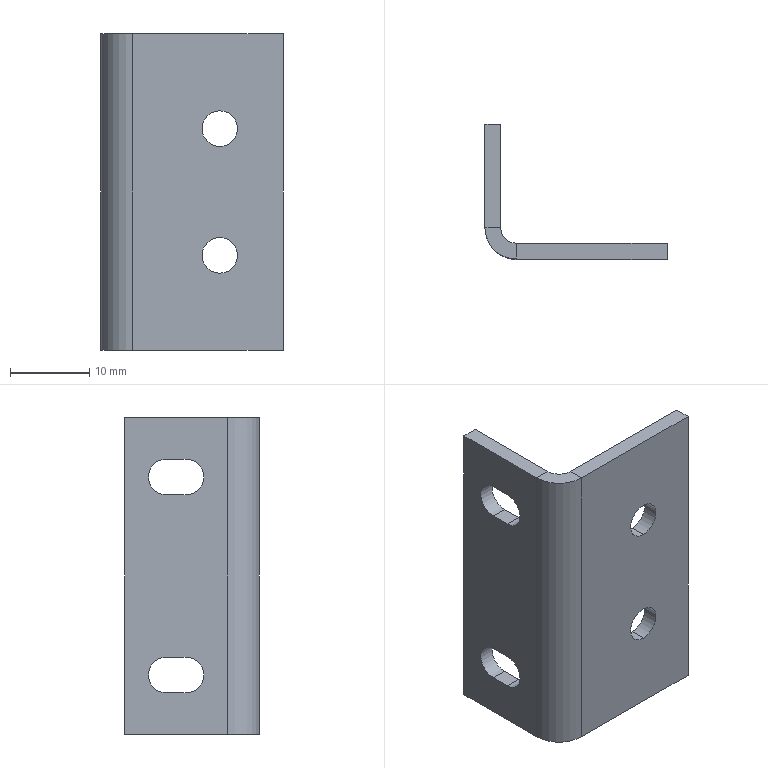Part | SolidWorks | features HoleWzd 2, FlatPattern 1, SMBaseFlange 1, SheetMetal 1 | 1 solid | 26 faces | box 23 x 17 x 40 mm | volume 2765 mm3 | plane 16 | cylinder 10 | commonest cylinder face diameters 4.5 x8 4 x1 8 x1
STEP:
#1=CARTESIAN_POINT('',(15.,-17.,9.75));
#2=VERTEX_POINT('',#1);
#3=CARTESIAN_POINT('',(15.,-17.,14.25));
#4=VERTEX_POINT('',#3);
#5=CARTESIAN_POINT('',(15.,-17.,12.));
#6=DIRECTION('',(0.,1.,0.));
#7=DIRECTION('',(0.,0.,1.));
#8=AXIS2_PLACEMENT_3D('',#5,#6,#7);
#9=CIRCLE('',#8,2.25);
#10=EDGE_CURVE('',#2,#4,#9,.T.);
#11=ORIENTED_EDGE('',*,*,#10,.F.);
#12=CARTESIAN_POINT('',(15.,-15.,9.75));
#13=VERTEX_POINT('',#12);
#14=CARTESIAN_POINT('',(15.,-15.,9.75));
#15=DIRECTION('',(0.,1.,0.));
#16=VECTOR('',#15,1000.);
#17=LINE('',#14,#16);
#18=EDGE_CURVE('',#2,#13,#17,.T.);
#19=ORIENTED_EDGE('',*,*,#18,.T.);
#20=CARTESIAN_POINT('',(15.,-15.,14.25));
#21=VERTEX_POINT('',#20);
#22=CARTESIAN_POINT('',(15.,-15.,12.));
#23=DIRECTION('',(0.,1.,0.));
#24=DIRECTION('',(0.,0.,1.));
#25=AXIS2_PLACEMENT_3D('',#22,#23,#24);
#26=CIRCLE('',#25,2.25);
#27=EDGE_CURVE('',#13,#21,#26,.T.);
#28=ORIENTED_EDGE('',*,*,#27,.T.);
#29=CARTESIAN_POINT('',(15.,-15.,14.25));
#30=DIRECTION('',(0.,1.,0.));
#31=VECTOR('',#30,1000.);
#32=LINE('',#29,#31);
#33=EDGE_CURVE('',#4,#21,#32,.T.);
#34=ORIENTED_EDGE('',*,*,#33,.F.);
#35=EDGE_LOOP('',(#11,#19,#28,#34));
#36=FACE_OUTER_BOUND('',#35,.T.);
#37=CARTESIAN_POINT('',(15.,-15.,12.));
#38=DIRECTION('',(0.,1.,0.));
#39=DIRECTION('',(0.,0.,1.));
#40=AXIS2_PLACEMENT_3D('',#37,#38,#39);
#41=CYLINDRICAL_SURFACE('',#40,2.25);
#42=ADVANCED_FACE('',(#36),#41,.F.);
#43=CARTESIAN_POINT('',(15.,-17.,25.75));
#44=VERTEX_POINT('',#43);
#45=CARTESIAN_POINT('',(15.,-17.,30.25));
#46=VERTEX_POINT('',#45);
#47=CARTESIAN_POINT('',(15.,-17.,28.));
#48=DIRECTION('',(0.,1.,0.));
#49=DIRECTION('',(0.,0.,1.));
#50=AXIS2_PLACEMENT_3D('',#47,#48,#49);
#51=CIRCLE('',#50,2.25);
#52=EDGE_CURVE('',#44,#46,#51,.T.);
#53=ORIENTED_EDGE('',*,*,#52,.F.);
#54=CARTESIAN_POINT('',(15.,-15.,25.75));
#55=VERTEX_POINT('',#54);
#56=CARTESIAN_POINT('',(15.,-15.,25.75));
#57=DIRECTION('',(0.,1.,0.));
#58=VECTOR('',#57,1000.);
#59=LINE('',#56,#58);
#60=EDGE_CURVE('',#44,#55,#59,.T.);
#61=ORIENTED_EDGE('',*,*,#60,.T.);
#62=CARTESIAN_POINT('',(15.,-15.,30.25));
#63=VERTEX_POINT('',#62);
#64=CARTESIAN_POINT('',(15.,-15.,28.));
#65=DIRECTION('',(0.,1.,0.));
#66=DIRECTION('',(0.,0.,1.));
#67=AXIS2_PLACEMENT_3D('',#64,#65,#66);
#68=CIRCLE('',#67,2.25);
#69=EDGE_CURVE('',#55,#63,#68,.T.);
#70=ORIENTED_EDGE('',*,*,#69,.T.);
#71=CARTESIAN_POINT('',(15.,-15.,30.25));
#72=DIRECTION('',(0.,1.,0.));
#73=VECTOR('',#72,1000.);
#74=LINE('',#71,#73);
#75=EDGE_CURVE('',#46,#63,#74,.T.);
#76=ORIENTED_EDGE('',*,*,#75,.F.);
#77=EDGE_LOOP('',(#53,#61,#70,#76));
#78=FACE_OUTER_BOUND('',#77,.T.);
#79=CARTESIAN_POINT('',(15.,-15.,28.));
#80=DIRECTION('',(0.,1.,0.));
#81=DIRECTION('',(0.,0.,1.));
#82=AXIS2_PLACEMENT_3D('',#79,#80,#81);
#83=CYLINDRICAL_SURFACE('',#82,2.25);
#84=ADVANCED_FACE('',(#78),#83,.F.);
#85=CARTESIAN_POINT('',(0.,-13.,40.));
#86=VERTEX_POINT('',#85);
#87=CARTESIAN_POINT('',(2.,-13.,40.));
#88=VERTEX_POINT('',#87);
#89=CARTESIAN_POINT('',(0.,-13.,40.));
#90=DIRECTION('',(1.,0.,0.));
#91=VECTOR('',#90,1000.);
#92=LINE('',#89,#91);
#93=EDGE_CURVE('',#86,#88,#92,.T.);
#94=ORIENTED_EDGE('',*,*,#93,.F.);
#95=CARTESIAN_POINT('',(4.,-17.,40.));
#96=VERTEX_POINT('',#95);
#97=CARTESIAN_POINT('',(4.,-13.,40.));
#98=DIRECTION('',(0.,0.,1.));
#99=DIRECTION('',(-1.,0.,0.));
#100=AXIS2_PLACEMENT_3D('',#97,#98,#99);
#101=CIRCLE('',#100,4.);
#102=EDGE_CURVE('',#86,#96,#101,.T.);
#103=ORIENTED_EDGE('',*,*,#102,.T.);
#104=CARTESIAN_POINT('',(4.,-15.,40.));
#105=VERTEX_POINT('',#104);
#106=CARTESIAN_POINT('',(4.,-15.,40.));
#107=DIRECTION('',(0.,-1.,0.));
#108=VECTOR('',#107,1000.);
#109=LINE('',#106,#108);
#110=EDGE_CURVE('',#105,#96,#109,.T.);
#111=ORIENTED_EDGE('',*,*,#110,.F.);
#112=CARTESIAN_POINT('',(4.,-13.,40.));
#113=DIRECTION('',(0.,0.,1.));
#114=DIRECTION('',(1.,0.,0.));
#115=AXIS2_PLACEMENT_3D('',#112,#113,#114);
#116=CIRCLE('',#115,2.);
#117=EDGE_CURVE('',#88,#105,#116,.T.);
#118=ORIENTED_EDGE('',*,*,#117,.F.);
#119=EDGE_LOOP('',(#94,#103,#111,#118));
#120=FACE_OUTER_BOUND('',#119,.T.);
#121=CARTESIAN_POINT('',(0.,-13.,40.));
#122=DIRECTION('',(0.,0.,1.));
#123=DIRECTION('',(1.,0.,0.));
#124=AXIS2_PLACEMENT_3D('',#121,#122,#123);
#125=PLANE('',#124);
#126=ADVANCED_FACE('',(#120),#125,.T.);
#127=CARTESIAN_POINT('',(0.,0.,40.));
#128=VERTEX_POINT('',#127);
#129=CARTESIAN_POINT('',(0.,0.,40.));
#130=DIRECTION('',(0.,-1.,0.));
#131=VECTOR('',#130,1000.);
#132=LINE('',#129,#131);
#133=EDGE_CURVE('',#128,#86,#132,.T.);
#134=ORIENTED_EDGE('',*,*,#133,.T.);
#135=ORIENTED_EDGE('',*,*,#93,.T.);
#136=CARTESIAN_POINT('',(2.,0.,40.));
#137=VERTEX_POINT('',#136);
#138=CARTESIAN_POINT('',(2.,0.,40.));
#139=DIRECTION('',(0.,-1.,0.));
#140=VECTOR('',#139,1000.);
#141=LINE('',#138,#140);
#142=EDGE_CURVE('',#137,#88,#141,.T.);
#143=ORIENTED_EDGE('',*,*,#142,.F.);
#144=CARTESIAN_POINT('',(0.,0.,40.));
#145=DIRECTION('',(1.,0.,0.));
#146=VECTOR('',#145,1000.);
#147=LINE('',#144,#146);
#148=EDGE_CURVE('',#128,#137,#147,.T.);
#149=ORIENTED_EDGE('',*,*,#148,.F.);
#150=EDGE_LOOP('',(#134,#135,#143,#149));
#151=FACE_OUTER_BOUND('',#150,.T.);
#152=CARTESIAN_POINT('',(4.,-15.,40.));
#153=DIRECTION('',(0.,0.,1.));
#154=DIRECTION('',(1.,0.,0.));
#155=AXIS2_PLACEMENT_3D('',#152,#153,#154);
#156=PLANE('',#155);
#157=ADVANCED_FACE('',(#151),#156,.T.);
#158=CARTESIAN_POINT('',(4.,-17.,0.));
#159=VERTEX_POINT('',#158);
#160=CARTESIAN_POINT('',(4.,-15.,0.));
#161=VERTEX_POINT('',#160);
#162=CARTESIAN_POINT('',(4.,-17.,0.));
#163=DIRECTION('',(0.,1.,0.));
#164=VECTOR('',#163,1000.);
#165=LINE('',#162,#164);
#166=EDGE_CURVE('',#159,#161,#165,.T.);
#167=ORIENTED_EDGE('',*,*,#166,.F.);
#168=CARTESIAN_POINT('',(0.,-13.,0.));
#169=VERTEX_POINT('',#168);
#170=CARTESIAN_POINT('',(4.,-13.,0.));
#171=DIRECTION('',(0.,0.,1.));
#172=DIRECTION('',(-1.,0.,0.));
#173=AXIS2_PLACEMENT_3D('',#170,#171,#172);
#174=CIRCLE('',#173,4.);
#175=EDGE_CURVE('',#169,#159,#174,.T.);
#176=ORIENTED_EDGE('',*,*,#175,.F.);
#177=CARTESIAN_POINT('',(2.,-13.,0.));
#178=VERTEX_POINT('',#177);
#179=CARTESIAN_POINT('',(2.,-13.,0.));
#180=DIRECTION('',(-1.,0.,0.));
#181=VECTOR('',#180,1000.);
#182=LINE('',#179,#181);
#183=EDGE_CURVE('',#178,#169,#182,.T.);
#184=ORIENTED_EDGE('',*,*,#183,.F.);
#185=CARTESIAN_POINT('',(4.,-13.,0.));
#186=DIRECTION('',(0.,0.,1.));
#187=DIRECTION('',(1.,0.,0.));
#188=AXIS2_PLACEMENT_3D('',#185,#186,#187);
#189=CIRCLE('',#188,2.);
#190=EDGE_CURVE('',#178,#161,#189,.T.);
#191=ORIENTED_EDGE('',*,*,#190,.T.);
#192=EDGE_LOOP('',(#167,#176,#184,#191));
#193=FACE_OUTER_BOUND('',#192,.T.);
#194=CARTESIAN_POINT('',(4.,-17.,0.));
#195=DIRECTION('',(0.,0.,-1.));
#196=DIRECTION('',(-1.,0.,0.));
#197=AXIS2_PLACEMENT_3D('',#194,#195,#196);
#198=PLANE('',#197);
#199=ADVANCED_FACE('',(#193),#198,.T.);
#200=CARTESIAN_POINT('',(23.,-17.,0.));
#201=VERTEX_POINT('',#200);
#202=CARTESIAN_POINT('',(0.,-17.,0.));
#203=DIRECTION('',(1.,0.,0.));
#204=VECTOR('',#203,1000.);
#205=LINE('',#202,#204);
#206=EDGE_CURVE('',#159,#201,#205,.T.);
#207=ORIENTED_EDGE('',*,*,#206,.F.);
#208=ORIENTED_EDGE('',*,*,#166,.T.);
#209=CARTESIAN_POINT('',(23.,-15.,0.));
#210=VERTEX_POINT('',#209);
#211=CARTESIAN_POINT('',(0.,-15.,0.));
#212=DIRECTION('',(1.,0.,0.));
#213=VECTOR('',#212,1000.);
#214=LINE('',#211,#213);
#215=EDGE_CURVE('',#161,#210,#214,.T.);
#216=ORIENTED_EDGE('',*,*,#215,.T.);
#217=CARTESIAN_POINT('',(23.,-15.,0.));
#218=DIRECTION('',(0.,-1.,0.));
#219=VECTOR('',#218,1000.);
#220=LINE('',#217,#219);
#221=EDGE_CURVE('',#210,#201,#220,.T.);
#222=ORIENTED_EDGE('',*,*,#221,.T.);
#223=EDGE_LOOP('',(#207,#208,#216,#222));
#224=FACE_OUTER_BOUND('',#223,.T.);
#225=CARTESIAN_POINT('',(2.,-13.,0.));
#226=DIRECTION('',(0.,0.,-1.));
#227=DIRECTION('',(-1.,0.,0.));
#228=AXIS2_PLACEMENT_3D('',#225,#226,#227);
#229=PLANE('',#228);
#230=ADVANCED_FACE('',(#224),#229,.T.);
#231=CARTESIAN_POINT('',(15.,-17.,12.));
#232=DIRECTION('',(0.,1.,0.));
#233=DIRECTION('',(0.,0.,1.));
#234=AXIS2_PLACEMENT_3D('',#231,#232,#233);
#235=CIRCLE('',#234,2.25);
#236=EDGE_CURVE('',#4,#2,#235,.T.);
#237=ORIENTED_EDGE('',*,*,#236,.T.);
#238=ORIENTED_EDGE('',*,*,#10,.T.);
#239=EDGE_LOOP('',(#237,#238));
#240=FACE_BOUND('',#239,.T.);
#241=CARTESIAN_POINT('',(15.,-17.,28.));
#242=DIRECTION('',(0.,1.,0.));
#243=DIRECTION('',(0.,0.,1.));
#244=AXIS2_PLACEMENT_3D('',#241,#242,#243);
#245=CIRCLE('',#244,2.25);
#246=EDGE_CURVE('',#46,#44,#245,.T.);
#247=ORIENTED_EDGE('',*,*,#246,.T.);
#248=ORIENTED_EDGE('',*,*,#52,.T.);
#249=EDGE_LOOP('',(#247,#248));
#250=FACE_BOUND('',#249,.T.);
#251=ORIENTED_EDGE('',*,*,#206,.T.);
#252=CARTESIAN_POINT('',(23.,-17.,40.));
#253=VERTEX_POINT('',#252);
#254=CARTESIAN_POINT('',(23.,-17.,40.));
#255=DIRECTION('',(0.,0.,-1.));
#256=VECTOR('',#255,1000.);
#257=LINE('',#254,#256);
#258=EDGE_CURVE('',#253,#201,#257,.T.);
#259=ORIENTED_EDGE('',*,*,#258,.F.);
#260=CARTESIAN_POINT('',(0.,-17.,40.));
#261=DIRECTION('',(1.,0.,0.));
#262=VECTOR('',#261,1000.);
#263=LINE('',#260,#262);
#264=EDGE_CURVE('',#96,#253,#263,.T.);
#265=ORIENTED_EDGE('',*,*,#264,.F.);
#266=CARTESIAN_POINT('',(4.,-17.,40.));
#267=DIRECTION('',(0.,0.,-1.));
#268=VECTOR('',#267,1000.);
#269=LINE('',#266,#268);
#270=EDGE_CURVE('',#96,#159,#269,.T.);
#271=ORIENTED_EDGE('',*,*,#270,.T.);
#272=EDGE_LOOP('',(#251,#259,#265,#271));
#273=FACE_OUTER_BOUND('',#272,.T.);
#274=CARTESIAN_POINT('',(0.,-17.,40.));
#275=DIRECTION('',(0.,1.,0.));
#276=DIRECTION('',(0.,0.,1.));
#277=AXIS2_PLACEMENT_3D('',#274,#275,#276);
#278=PLANE('',#277);
#279=ADVANCED_FACE('',(#240,#250,#273),#278,.F.);
#280=ORIENTED_EDGE('',*,*,#221,.F.);
#281=CARTESIAN_POINT('',(23.,-15.,40.));
#282=VERTEX_POINT('',#281);
#283=CARTESIAN_POINT('',(23.,-15.,40.));
#284=DIRECTION('',(0.,0.,-1.));
#285=VECTOR('',#284,1000.);
#286=LINE('',#283,#285);
#287=EDGE_CURVE('',#282,#210,#286,.T.);
#288=ORIENTED_EDGE('',*,*,#287,.F.);
#289=CARTESIAN_POINT('',(23.,-15.,40.));
#290=DIRECTION('',(0.,-1.,0.));
#291=VECTOR('',#290,1000.);
#292=LINE('',#289,#291);
#293=EDGE_CURVE('',#282,#253,#292,.T.);
#294=ORIENTED_EDGE('',*,*,#293,.T.);
#295=ORIENTED_EDGE('',*,*,#258,.T.);
#296=EDGE_LOOP('',(#280,#288,#294,#295));
#297=FACE_OUTER_BOUND('',#296,.T.);
#298=CARTESIAN_POINT('',(23.,-15.,40.));
#299=DIRECTION('',(1.,0.,0.));
#300=DIRECTION('',(0.,0.,-1.));
#301=AXIS2_PLACEMENT_3D('',#298,#299,#300);
#302=PLANE('',#301);
#303=ADVANCED_FACE('',(#297),#302,.T.);
#304=CARTESIAN_POINT('',(15.,-15.,12.));
#305=DIRECTION('',(0.,1.,0.));
#306=DIRECTION('',(0.,0.,1.));
#307=AXIS2_PLACEMENT_3D('',#304,#305,#306);
#308=CIRCLE('',#307,2.25);
#309=EDGE_CURVE('',#21,#13,#308,.T.);
#310=ORIENTED_EDGE('',*,*,#309,.F.);
#311=ORIENTED_EDGE('',*,*,#27,.F.);
#312=EDGE_LOOP('',(#310,#311));
#313=FACE_BOUND('',#312,.T.);
#314=CARTESIAN_POINT('',(15.,-15.,28.));
#315=DIRECTION('',(0.,1.,0.));
#316=DIRECTION('',(0.,0.,1.));
#317=AXIS2_PLACEMENT_3D('',#314,#315,#316);
#318=CIRCLE('',#317,2.25);
#319=EDGE_CURVE('',#63,#55,#318,.T.);
#320=ORIENTED_EDGE('',*,*,#319,.F.);
#321=ORIENTED_EDGE('',*,*,#69,.F.);
#322=EDGE_LOOP('',(#320,#321));
#323=FACE_BOUND('',#322,.T.);
#324=ORIENTED_EDGE('',*,*,#215,.F.);
#325=CARTESIAN_POINT('',(4.,-15.,40.));
#326=DIRECTION('',(0.,0.,-1.));
#327=VECTOR('',#326,1000.);
#328=LINE('',#325,#327);
#329=EDGE_CURVE('',#105,#161,#328,.T.);
#330=ORIENTED_EDGE('',*,*,#329,.F.);
#331=CARTESIAN_POINT('',(0.,-15.,40.));
#332=DIRECTION('',(1.,0.,0.));
#333=VECTOR('',#332,1000.);
#334=LINE('',#331,#333);
#335=EDGE_CURVE('',#105,#282,#334,.T.);
#336=ORIENTED_EDGE('',*,*,#335,.T.);
#337=ORIENTED_EDGE('',*,*,#287,.T.);
#338=EDGE_LOOP('',(#324,#330,#336,#337));
#339=FACE_OUTER_BOUND('',#338,.T.);
#340=CARTESIAN_POINT('',(0.,-15.,40.));
#341=DIRECTION('',(0.,1.,0.));
#342=DIRECTION('',(0.,0.,1.));
#343=AXIS2_PLACEMENT_3D('',#340,#341,#342);
#344=PLANE('',#343);
#345=ADVANCED_FACE('',(#313,#323,#339),#344,.T.);
#346=ORIENTED_EDGE('',*,*,#190,.F.);
#347=CARTESIAN_POINT('',(2.,-13.,40.));
#348=DIRECTION('',(0.,0.,-1.));
#349=VECTOR('',#348,1000.);
#350=LINE('',#347,#349);
#351=EDGE_CURVE('',#88,#178,#350,.T.);
#352=ORIENTED_EDGE('',*,*,#351,.F.);
#353=ORIENTED_EDGE('',*,*,#117,.T.);
#354=ORIENTED_EDGE('',*,*,#329,.T.);
#355=EDGE_LOOP('',(#346,#352,#353,#354));
#356=FACE_OUTER_BOUND('',#355,.T.);
#357=CARTESIAN_POINT('',(4.,-13.,40.));
#358=DIRECTION('',(0.,0.,-1.));
#359=DIRECTION('',(-1.,0.,0.));
#360=AXIS2_PLACEMENT_3D('',#357,#358,#359);
#361=CYLINDRICAL_SURFACE('',#360,2.);
#362=ADVANCED_FACE('',(#356),#361,.F.);
#363=CARTESIAN_POINT('',(2.,-7.75,9.75));
#364=VERTEX_POINT('',#363);
#365=CARTESIAN_POINT('',(2.,-7.75,5.25));
#366=VERTEX_POINT('',#365);
#367=CARTESIAN_POINT('',(2.,-7.75,7.5));
#368=DIRECTION('',(1.,0.,0.));
#369=DIRECTION('',(0.,0.,-1.));
#370=AXIS2_PLACEMENT_3D('',#367,#368,#369);
#371=CIRCLE('',#370,2.25);
#372=EDGE_CURVE('',#364,#366,#371,.T.);
#373=ORIENTED_EDGE('',*,*,#372,.F.);
#374=CARTESIAN_POINT('',(2.,-5.25,9.75));
#375=VERTEX_POINT('',#374);
#376=CARTESIAN_POINT('',(2.,-7.75,9.75));
#377=DIRECTION('',(0.,1.,0.));
#378=VECTOR('',#377,1000.);
#379=LINE('',#376,#378);
#380=EDGE_CURVE('',#364,#375,#379,.T.);
#381=ORIENTED_EDGE('',*,*,#380,.T.);
#382=CARTESIAN_POINT('',(2.,-5.25,5.25));
#383=VERTEX_POINT('',#382);
#384=CARTESIAN_POINT('',(2.,-5.25,7.5));
#385=DIRECTION('',(1.,0.,0.));
#386=DIRECTION('',(0.,0.,-1.));
#387=AXIS2_PLACEMENT_3D('',#384,#385,#386);
#388=CIRCLE('',#387,2.25);
#389=EDGE_CURVE('',#383,#375,#388,.T.);
#390=ORIENTED_EDGE('',*,*,#389,.F.);
#391=CARTESIAN_POINT('',(2.,-7.75,5.25));
#392=DIRECTION('',(0.,1.,0.));
#393=VECTOR('',#392,1000.);
#394=LINE('',#391,#393);
#395=EDGE_CURVE('',#366,#383,#394,.T.);
#396=ORIENTED_EDGE('',*,*,#395,.F.);
#397=EDGE_LOOP('',(#373,#381,#390,#396));
#398=FACE_BOUND('',#397,.T.);
#399=CARTESIAN_POINT('',(2.,-5.25,30.25));
#400=VERTEX_POINT('',#399);
#401=CARTESIAN_POINT('',(2.,-5.25,34.75));
#402=VERTEX_POINT('',#401);
#403=CARTESIAN_POINT('',(2.,-5.25,32.5));
#404=DIRECTION('',(1.,0.,0.));
#405=DIRECTION('',(0.,0.,-1.));
#406=AXIS2_PLACEMENT_3D('',#403,#404,#405);
#407=CIRCLE('',#406,2.25);
#408=EDGE_CURVE('',#400,#402,#407,.T.);
#409=ORIENTED_EDGE('',*,*,#408,.F.);
#410=CARTESIAN_POINT('',(2.,-7.75,30.25));
#411=VERTEX_POINT('',#410);
#412=CARTESIAN_POINT('',(2.,-7.75,30.25));
#413=DIRECTION('',(0.,1.,0.));
#414=VECTOR('',#413,1000.);
#415=LINE('',#412,#414);
#416=EDGE_CURVE('',#411,#400,#415,.T.);
#417=ORIENTED_EDGE('',*,*,#416,.F.);
#418=CARTESIAN_POINT('',(2.,-7.75,34.75));
#419=VERTEX_POINT('',#418);
#420=CARTESIAN_POINT('',(2.,-7.75,32.5));
#421=DIRECTION('',(1.,0.,0.));
#422=DIRECTION('',(0.,0.,-1.));
#423=AXIS2_PLACEMENT_3D('',#420,#421,#422);
#424=CIRCLE('',#423,2.25);
#425=EDGE_CURVE('',#419,#411,#424,.T.);
#426=ORIENTED_EDGE('',*,*,#425,.F.);
#427=CARTESIAN_POINT('',(2.,-7.75,34.75));
#428=DIRECTION('',(0.,1.,0.));
#429=VECTOR('',#428,1000.);
#430=LINE('',#427,#429);
#431=EDGE_CURVE('',#419,#402,#430,.T.);
#432=ORIENTED_EDGE('',*,*,#431,.T.);
#433=EDGE_LOOP('',(#409,#417,#426,#432));
#434=FACE_BOUND('',#433,.T.);
#435=CARTESIAN_POINT('',(2.,0.,0.));
#436=VERTEX_POINT('',#435);
#437=CARTESIAN_POINT('',(2.,0.,0.));
#438=DIRECTION('',(0.,-1.,0.));
#439=VECTOR('',#438,1000.);
#440=LINE('',#437,#439);
#441=EDGE_CURVE('',#436,#178,#440,.T.);
#442=ORIENTED_EDGE('',*,*,#441,.F.);
#443=CARTESIAN_POINT('',(2.,0.,40.));
#444=DIRECTION('',(0.,0.,-1.));
#445=VECTOR('',#444,1000.);
#446=LINE('',#443,#445);
#447=EDGE_CURVE('',#137,#436,#446,.T.);
#448=ORIENTED_EDGE('',*,*,#447,.F.);
#449=ORIENTED_EDGE('',*,*,#142,.T.);
#450=ORIENTED_EDGE('',*,*,#351,.T.);
#451=EDGE_LOOP('',(#442,#448,#449,#450));
#452=FACE_OUTER_BOUND('',#451,.T.);
#453=CARTESIAN_POINT('',(2.,0.,40.));
#454=DIRECTION('',(1.,0.,0.));
#455=DIRECTION('',(0.,1.,0.));
#456=AXIS2_PLACEMENT_3D('',#453,#454,#455);
#457=PLANE('',#456);
#458=ADVANCED_FACE('',(#398,#434,#452),#457,.T.);
#459=CARTESIAN_POINT('',(0.,0.,0.));
#460=VERTEX_POINT('',#459);
#461=CARTESIAN_POINT('',(0.,0.,0.));
#462=DIRECTION('',(1.,0.,0.));
#463=VECTOR('',#462,1000.);
#464=LINE('',#461,#463);
#465=EDGE_CURVE('',#460,#436,#464,.T.);
#466=ORIENTED_EDGE('',*,*,#465,.F.);
#467=CARTESIAN_POINT('',(0.,0.,40.));
#468=DIRECTION('',(0.,0.,-1.));
#469=VECTOR('',#468,1000.);
#470=LINE('',#467,#469);
#471=EDGE_CURVE('',#128,#460,#470,.T.);
#472=ORIENTED_EDGE('',*,*,#471,.F.);
#473=ORIENTED_EDGE('',*,*,#148,.T.);
#474=ORIENTED_EDGE('',*,*,#447,.T.);
#475=EDGE_LOOP('',(#466,#472,#473,#474));
#476=FACE_OUTER_BOUND('',#475,.T.);
#477=CARTESIAN_POINT('',(0.,0.,40.));
#478=DIRECTION('',(0.,1.,0.));
#479=DIRECTION('',(-1.,0.,0.));
#480=AXIS2_PLACEMENT_3D('',#477,#478,#479);
#481=PLANE('',#480);
#482=ADVANCED_FACE('',(#476),#481,.T.);
#483=CARTESIAN_POINT('',(0.,-7.75,9.75));
#484=VERTEX_POINT('',#483);
#485=CARTESIAN_POINT('',(0.,-7.75,5.25));
#486=VERTEX_POINT('',#485);
#487=CARTESIAN_POINT('',(0.,-7.75,7.5));
#488=DIRECTION('',(1.,0.,0.));
#489=DIRECTION('',(0.,1.,0.));
#490=AXIS2_PLACEMENT_3D('',#487,#488,#489);
#491=CIRCLE('',#490,2.25);
#492=EDGE_CURVE('',#484,#486,#491,.T.);
#493=ORIENTED_EDGE('',*,*,#492,.T.);
#494=CARTESIAN_POINT('',(0.,-5.25,5.25));
#495=VERTEX_POINT('',#494);
#496=CARTESIAN_POINT('',(0.,0.,5.25));
#497=DIRECTION('',(0.,1.,0.));
#498=VECTOR('',#497,1000.);
#499=LINE('',#496,#498);
#500=EDGE_CURVE('',#486,#495,#499,.T.);
#501=ORIENTED_EDGE('',*,*,#500,.T.);
#502=CARTESIAN_POINT('',(0.,-5.25,9.75));
#503=VERTEX_POINT('',#502);
#504=CARTESIAN_POINT('',(0.,-5.25,7.5));
#505=DIRECTION('',(1.,0.,0.));
#506=DIRECTION('',(0.,1.,0.));
#507=AXIS2_PLACEMENT_3D('',#504,#505,#506);
#508=CIRCLE('',#507,2.25);
#509=EDGE_CURVE('',#495,#503,#508,.T.);
#510=ORIENTED_EDGE('',*,*,#509,.T.);
#511=CARTESIAN_POINT('',(0.,0.,9.75));
#512=DIRECTION('',(0.,-1.,0.));
#513=VECTOR('',#512,1000.);
#514=LINE('',#511,#513);
#515=EDGE_CURVE('',#503,#484,#514,.T.);
#516=ORIENTED_EDGE('',*,*,#515,.T.);
#517=EDGE_LOOP('',(#493,#501,#510,#516));
#518=FACE_BOUND('',#517,.T.);
#519=CARTESIAN_POINT('',(0.,-5.25,30.25));
#520=VERTEX_POINT('',#519);
#521=CARTESIAN_POINT('',(0.,-5.25,34.75));
#522=VERTEX_POINT('',#521);
#523=CARTESIAN_POINT('',(0.,-5.25,32.5));
#524=DIRECTION('',(1.,0.,0.));
#525=DIRECTION('',(0.,1.,0.));
#526=AXIS2_PLACEMENT_3D('',#523,#524,#525);
#527=CIRCLE('',#526,2.25);
#528=EDGE_CURVE('',#520,#522,#527,.T.);
#529=ORIENTED_EDGE('',*,*,#528,.T.);
#530=CARTESIAN_POINT('',(0.,-7.75,34.75));
#531=VERTEX_POINT('',#530);
#532=CARTESIAN_POINT('',(0.,0.,34.75));
#533=DIRECTION('',(0.,-1.,0.));
#534=VECTOR('',#533,1000.);
#535=LINE('',#532,#534);
#536=EDGE_CURVE('',#522,#531,#535,.T.);
#537=ORIENTED_EDGE('',*,*,#536,.T.);
#538=CARTESIAN_POINT('',(0.,-7.75,30.25));
#539=VERTEX_POINT('',#538);
#540=CARTESIAN_POINT('',(0.,-7.75,32.5));
#541=DIRECTION('',(1.,0.,0.));
#542=DIRECTION('',(0.,1.,0.));
#543=AXIS2_PLACEMENT_3D('',#540,#541,#542);
#544=CIRCLE('',#543,2.25);
#545=EDGE_CURVE('',#531,#539,#544,.T.);
#546=ORIENTED_EDGE('',*,*,#545,.T.);
#547=CARTESIAN_POINT('',(0.,0.,30.25));
#548=DIRECTION('',(0.,1.,0.));
#549=VECTOR('',#548,1000.);
#550=LINE('',#547,#549);
#551=EDGE_CURVE('',#539,#520,#550,.T.);
#552=ORIENTED_EDGE('',*,*,#551,.T.);
#553=EDGE_LOOP('',(#529,#537,#546,#552));
#554=FACE_BOUND('',#553,.T.);
#555=CARTESIAN_POINT('',(0.,0.,0.));
#556=DIRECTION('',(0.,-1.,0.));
#557=VECTOR('',#556,1000.);
#558=LINE('',#555,#557);
#559=EDGE_CURVE('',#460,#169,#558,.T.);
#560=ORIENTED_EDGE('',*,*,#559,.T.);
#561=CARTESIAN_POINT('',(0.,-13.,40.));
#562=DIRECTION('',(0.,0.,-1.));
#563=VECTOR('',#562,1000.);
#564=LINE('',#561,#563);
#565=EDGE_CURVE('',#86,#169,#564,.T.);
#566=ORIENTED_EDGE('',*,*,#565,.F.);
#567=ORIENTED_EDGE('',*,*,#133,.F.);
#568=ORIENTED_EDGE('',*,*,#471,.T.);
#569=EDGE_LOOP('',(#560,#566,#567,#568));
#570=FACE_OUTER_BOUND('',#569,.T.);
#571=CARTESIAN_POINT('',(0.,0.,40.));
#572=DIRECTION('',(1.,0.,0.));
#573=DIRECTION('',(0.,1.,0.));
#574=AXIS2_PLACEMENT_3D('',#571,#572,#573);
#575=PLANE('',#574);
#576=ADVANCED_FACE('',(#518,#554,#570),#575,.F.);
#577=ORIENTED_EDGE('',*,*,#175,.T.);
#578=ORIENTED_EDGE('',*,*,#270,.F.);
#579=ORIENTED_EDGE('',*,*,#102,.F.);
#580=ORIENTED_EDGE('',*,*,#565,.T.);
#581=EDGE_LOOP('',(#577,#578,#579,#580));
#582=FACE_OUTER_BOUND('',#581,.T.);
#583=CARTESIAN_POINT('',(4.,-13.,40.));
#584=DIRECTION('',(0.,0.,-1.));
#585=DIRECTION('',(-1.,0.,0.));
#586=AXIS2_PLACEMENT_3D('',#583,#584,#585);
#587=CYLINDRICAL_SURFACE('',#586,4.);
#588=ADVANCED_FACE('',(#582),#587,.T.);
#589=ORIENTED_EDGE('',*,*,#264,.T.);
#590=ORIENTED_EDGE('',*,*,#293,.F.);
#591=ORIENTED_EDGE('',*,*,#335,.F.);
#592=ORIENTED_EDGE('',*,*,#110,.T.);
#593=EDGE_LOOP('',(#589,#590,#591,#592));
#594=FACE_OUTER_BOUND('',#593,.T.);
#595=CARTESIAN_POINT('',(4.,-13.,40.));
#596=DIRECTION('',(0.,0.,1.));
#597=DIRECTION('',(1.,0.,0.));
#598=AXIS2_PLACEMENT_3D('',#595,#596,#597);
#599=PLANE('',#598);
#600=ADVANCED_FACE('',(#594),#599,.T.);
#601=ORIENTED_EDGE('',*,*,#441,.T.);
#602=ORIENTED_EDGE('',*,*,#183,.T.);
#603=ORIENTED_EDGE('',*,*,#559,.F.);
#604=ORIENTED_EDGE('',*,*,#465,.T.);
#605=EDGE_LOOP('',(#601,#602,#603,#604));
#606=FACE_OUTER_BOUND('',#605,.T.);
#607=CARTESIAN_POINT('',(4.,-13.,0.));
#608=DIRECTION('',(0.,0.,1.));
#609=DIRECTION('',(1.,0.,0.));
#610=AXIS2_PLACEMENT_3D('',#607,#608,#609);
#611=PLANE('',#610);
#612=ADVANCED_FACE('',(#606),#611,.F.);
#613=ORIENTED_EDGE('',*,*,#60,.F.);
#614=ORIENTED_EDGE('',*,*,#246,.F.);
#615=ORIENTED_EDGE('',*,*,#75,.T.);
#616=ORIENTED_EDGE('',*,*,#319,.T.);
#617=EDGE_LOOP('',(#613,#614,#615,#616));
#618=FACE_OUTER_BOUND('',#617,.T.);
#619=CARTESIAN_POINT('',(15.,-15.,28.));
#620=DIRECTION('',(0.,1.,0.));
#621=DIRECTION('',(0.,0.,1.));
#622=AXIS2_PLACEMENT_3D('',#619,#620,#621);
#623=CYLINDRICAL_SURFACE('',#622,2.25);
#624=ADVANCED_FACE('',(#618),#623,.F.);
#625=ORIENTED_EDGE('',*,*,#18,.F.);
#626=ORIENTED_EDGE('',*,*,#236,.F.);
#627=ORIENTED_EDGE('',*,*,#33,.T.);
#628=ORIENTED_EDGE('',*,*,#309,.T.);
#629=EDGE_LOOP('',(#625,#626,#627,#628));
#630=FACE_OUTER_BOUND('',#629,.T.);
#631=CARTESIAN_POINT('',(15.,-15.,12.));
#632=DIRECTION('',(0.,1.,0.));
#633=DIRECTION('',(0.,0.,1.));
#634=AXIS2_PLACEMENT_3D('',#631,#632,#633);
#635=CYLINDRICAL_SURFACE('',#634,2.25);
#636=ADVANCED_FACE('',(#630),#635,.F.);
#637=CARTESIAN_POINT('',(2.,-7.75,34.75));
#638=DIRECTION('',(-1.,0.,0.));
#639=VECTOR('',#638,1000.);
#640=LINE('',#637,#639);
#641=EDGE_CURVE('',#419,#531,#640,.T.);
#642=ORIENTED_EDGE('',*,*,#641,.F.);
#643=ORIENTED_EDGE('',*,*,#425,.T.);
#644=CARTESIAN_POINT('',(2.,-7.75,30.25));
#645=DIRECTION('',(1.,0.,0.));
#646=VECTOR('',#645,1000.);
#647=LINE('',#644,#646);
#648=EDGE_CURVE('',#539,#411,#647,.T.);
#649=ORIENTED_EDGE('',*,*,#648,.F.);
#650=ORIENTED_EDGE('',*,*,#545,.F.);
#651=EDGE_LOOP('',(#642,#643,#649,#650));
#652=FACE_OUTER_BOUND('',#651,.T.);
#653=CARTESIAN_POINT('',(2.,-7.75,32.5));
#654=DIRECTION('',(1.,0.,0.));
#655=DIRECTION('',(0.,0.,-1.));
#656=AXIS2_PLACEMENT_3D('',#653,#654,#655);
#657=CYLINDRICAL_SURFACE('',#656,2.25);
#658=ADVANCED_FACE('',(#652),#657,.F.);
#659=CARTESIAN_POINT('',(2.,-5.25,30.25));
#660=DIRECTION('',(-1.,0.,0.));
#661=VECTOR('',#660,1000.);
#662=LINE('',#659,#661);
#663=EDGE_CURVE('',#400,#520,#662,.T.);
#664=ORIENTED_EDGE('',*,*,#663,.F.);
#665=ORIENTED_EDGE('',*,*,#408,.T.);
#666=CARTESIAN_POINT('',(2.,-5.25,34.75));
#667=DIRECTION('',(1.,0.,0.));
#668=VECTOR('',#667,1000.);
#669=LINE('',#666,#668);
#670=EDGE_CURVE('',#522,#402,#669,.T.);
#671=ORIENTED_EDGE('',*,*,#670,.F.);
#672=ORIENTED_EDGE('',*,*,#528,.F.);
#673=EDGE_LOOP('',(#664,#665,#671,#672));
#674=FACE_OUTER_BOUND('',#673,.T.);
#675=CARTESIAN_POINT('',(2.,-5.25,32.5));
#676=DIRECTION('',(1.,0.,0.));
#677=DIRECTION('',(0.,0.,-1.));
#678=AXIS2_PLACEMENT_3D('',#675,#676,#677);
#679=CYLINDRICAL_SURFACE('',#678,2.25);
#680=ADVANCED_FACE('',(#674),#679,.F.);
#681=ORIENTED_EDGE('',*,*,#670,.T.);
#682=ORIENTED_EDGE('',*,*,#431,.F.);
#683=ORIENTED_EDGE('',*,*,#641,.T.);
#684=ORIENTED_EDGE('',*,*,#536,.F.);
#685=EDGE_LOOP('',(#681,#682,#683,#684));
#686=FACE_OUTER_BOUND('',#685,.T.);
#687=CARTESIAN_POINT('',(2.,-7.75,34.75));
#688=DIRECTION('',(0.,0.,1.));
#689=DIRECTION('',(1.,0.,0.));
#690=AXIS2_PLACEMENT_3D('',#687,#688,#689);
#691=PLANE('',#690);
#692=ADVANCED_FACE('',(#686),#691,.F.);
#693=ORIENTED_EDGE('',*,*,#648,.T.);
#694=ORIENTED_EDGE('',*,*,#416,.T.);
#695=ORIENTED_EDGE('',*,*,#663,.T.);
#696=ORIENTED_EDGE('',*,*,#551,.F.);
#697=EDGE_LOOP('',(#693,#694,#695,#696));
#698=FACE_OUTER_BOUND('',#697,.T.);
#699=CARTESIAN_POINT('',(2.,-7.75,30.25));
#700=DIRECTION('',(0.,0.,-1.));
#701=DIRECTION('',(-1.,0.,0.));
#702=AXIS2_PLACEMENT_3D('',#699,#700,#701);
#703=PLANE('',#702);
#704=ADVANCED_FACE('',(#698),#703,.F.);
#705=CARTESIAN_POINT('',(2.,-7.75,9.75));
#706=DIRECTION('',(-1.,0.,0.));
#707=VECTOR('',#706,1000.);
#708=LINE('',#705,#707);
#709=EDGE_CURVE('',#364,#484,#708,.T.);
#710=ORIENTED_EDGE('',*,*,#709,.F.);
#711=ORIENTED_EDGE('',*,*,#372,.T.);
#712=CARTESIAN_POINT('',(2.,-7.75,5.25));
#713=DIRECTION('',(1.,0.,0.));
#714=VECTOR('',#713,1000.);
#715=LINE('',#712,#714);
#716=EDGE_CURVE('',#486,#366,#715,.T.);
#717=ORIENTED_EDGE('',*,*,#716,.F.);
#718=ORIENTED_EDGE('',*,*,#492,.F.);
#719=EDGE_LOOP('',(#710,#711,#717,#718));
#720=FACE_OUTER_BOUND('',#719,.T.);
#721=CARTESIAN_POINT('',(2.,-7.75,7.5));
#722=DIRECTION('',(1.,0.,0.));
#723=DIRECTION('',(0.,0.,-1.));
#724=AXIS2_PLACEMENT_3D('',#721,#722,#723);
#725=CYLINDRICAL_SURFACE('',#724,2.25);
#726=ADVANCED_FACE('',(#720),#725,.F.);
#727=ORIENTED_EDGE('',*,*,#716,.T.);
#728=ORIENTED_EDGE('',*,*,#395,.T.);
#729=CARTESIAN_POINT('',(2.,-5.25,5.25));
#730=DIRECTION('',(-1.,0.,0.));
#731=VECTOR('',#730,1000.);
#732=LINE('',#729,#731);
#733=EDGE_CURVE('',#383,#495,#732,.T.);
#734=ORIENTED_EDGE('',*,*,#733,.T.);
#735=ORIENTED_EDGE('',*,*,#500,.F.);
#736=EDGE_LOOP('',(#727,#728,#734,#735));
#737=FACE_OUTER_BOUND('',#736,.T.);
#738=CARTESIAN_POINT('',(2.,-7.75,5.25));
#739=DIRECTION('',(0.,0.,-1.));
#740=DIRECTION('',(-1.,0.,0.));
#741=AXIS2_PLACEMENT_3D('',#738,#739,#740);
#742=PLANE('',#741);
#743=ADVANCED_FACE('',(#737),#742,.F.);
#744=CARTESIAN_POINT('',(2.,-5.25,9.75));
#745=DIRECTION('',(1.,0.,0.));
#746=VECTOR('',#745,1000.);
#747=LINE('',#744,#746);
#748=EDGE_CURVE('',#503,#375,#747,.T.);
#749=ORIENTED_EDGE('',*,*,#748,.T.);
#750=ORIENTED_EDGE('',*,*,#380,.F.);
#751=ORIENTED_EDGE('',*,*,#709,.T.);
#752=ORIENTED_EDGE('',*,*,#515,.F.);
#753=EDGE_LOOP('',(#749,#750,#751,#752));
#754=FACE_OUTER_BOUND('',#753,.T.);
#755=CARTESIAN_POINT('',(2.,-7.75,9.75));
#756=DIRECTION('',(0.,0.,1.));
#757=DIRECTION('',(1.,0.,0.));
#758=AXIS2_PLACEMENT_3D('',#755,#756,#757);
#759=PLANE('',#758);
#760=ADVANCED_FACE('',(#754),#759,.F.);
#761=ORIENTED_EDGE('',*,*,#733,.F.);
#762=ORIENTED_EDGE('',*,*,#389,.T.);
#763=ORIENTED_EDGE('',*,*,#748,.F.);
#764=ORIENTED_EDGE('',*,*,#509,.F.);
#765=EDGE_LOOP('',(#761,#762,#763,#764));
#766=FACE_OUTER_BOUND('',#765,.T.);
#767=CARTESIAN_POINT('',(2.,-5.25,7.5));
#768=DIRECTION('',(1.,0.,0.));
#769=DIRECTION('',(0.,0.,-1.));
#770=AXIS2_PLACEMENT_3D('',#767,#768,#769);
#771=CYLINDRICAL_SURFACE('',#770,2.25);
#772=ADVANCED_FACE('',(#766),#771,.F.);
#773=CLOSED_SHELL('',(#42,#84,#126,#157,#199,#230,#279,#303,#345,#362,#458,#482,#576,#588,#600,#612,#624,#636,#658,#680,#692,#704,#726,#743,#760,#772));
#774=MANIFOLD_SOLID_BREP('',#773);
#775=CARTESIAN_POINT('',(0.,0.,0.));
#776=DIRECTION('',(0.,0.,1.));
#777=DIRECTION('',(1.,0.,0.));
#778=AXIS2_PLACEMENT_3D('',#775,#776,#777);
#779=(LENGTH_UNIT()NAMED_UNIT(*)SI_UNIT(.MILLI.,.METRE.));
#780=UNCERTAINTY_MEASURE_WITH_UNIT(LENGTH_MEASURE(0.00001),#779,'','');
#781=(NAMED_UNIT(*)PLANE_ANGLE_UNIT()SI_UNIT($,.RADIAN.));
#782=(NAMED_UNIT(*)SI_UNIT($,.STERADIAN.)SOLID_ANGLE_UNIT());
#783=(GEOMETRIC_REPRESENTATION_CONTEXT(3)GLOBAL_UNCERTAINTY_ASSIGNED_CONTEXT((#780))GLOBAL_UNIT_ASSIGNED_CONTEXT((#779,#781,#782))REPRESENTATION_CONTEXT('',''));
#784=ADVANCED_BREP_SHAPE_REPRESENTATION('',(#774,#778),#783);